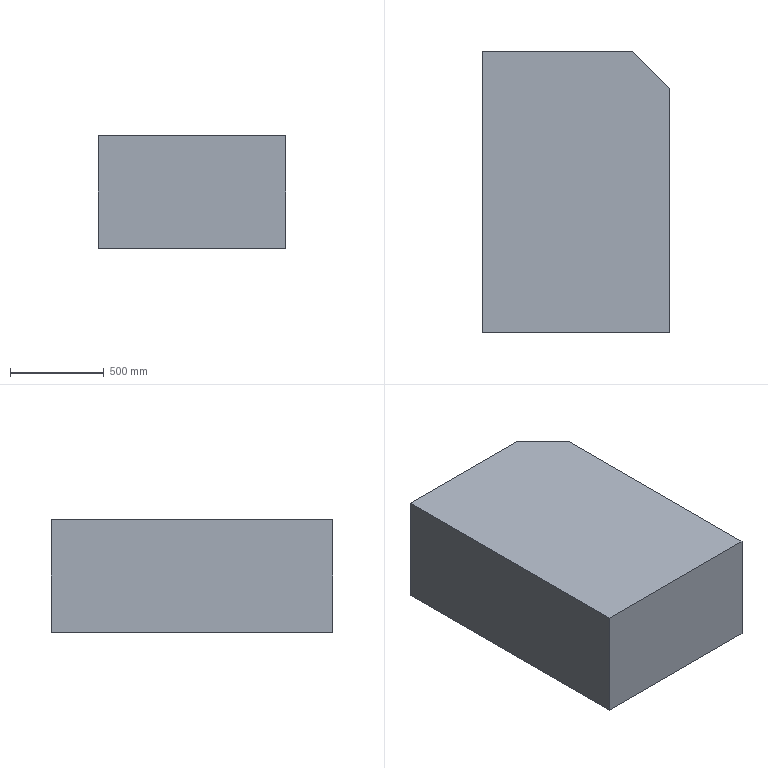Part | SolidWorks | features Chamfer 1, Extrusion 1 | 1 solid | 7 faces | box 1000 x 1500 x 600 mm | volume 888000000 mm3 | plane 7
STEP:
#1=CARTESIAN_POINT('',(500.,-750.,0.));
#2=VERTEX_POINT('',#1);
#3=CARTESIAN_POINT('',(500.,550.,0.));
#4=VERTEX_POINT('',#3);
#5=CARTESIAN_POINT('',(500.,750.,0.));
#6=DIRECTION('',(0.,1.,0.));
#7=VECTOR('',#6,1000.);
#8=LINE('',#5,#7);
#9=EDGE_CURVE('',#2,#4,#8,.T.);
#10=ORIENTED_EDGE('',*,*,#9,.T.);
#11=CARTESIAN_POINT('',(500.,550.,600.));
#12=VERTEX_POINT('',#11);
#13=CARTESIAN_POINT('',(500.,550.,600.));
#14=DIRECTION('',(0.,0.,1.));
#15=VECTOR('',#14,1000.);
#16=LINE('',#13,#15);
#17=EDGE_CURVE('',#4,#12,#16,.T.);
#18=ORIENTED_EDGE('',*,*,#17,.T.);
#19=CARTESIAN_POINT('',(500.,-750.,600.));
#20=VERTEX_POINT('',#19);
#21=CARTESIAN_POINT('',(500.,750.,600.));
#22=DIRECTION('',(0.,1.,0.));
#23=VECTOR('',#22,1000.);
#24=LINE('',#21,#23);
#25=EDGE_CURVE('',#20,#12,#24,.T.);
#26=ORIENTED_EDGE('',*,*,#25,.F.);
#27=CARTESIAN_POINT('',(500.,-750.,600.));
#28=DIRECTION('',(0.,0.,-1.));
#29=VECTOR('',#28,1000.);
#30=LINE('',#27,#29);
#31=EDGE_CURVE('',#20,#2,#30,.T.);
#32=ORIENTED_EDGE('',*,*,#31,.T.);
#33=EDGE_LOOP('',(#10,#18,#26,#32));
#34=FACE_OUTER_BOUND('',#33,.T.);
#35=CARTESIAN_POINT('',(500.,750.,600.));
#36=DIRECTION('',(-1.,0.,0.));
#37=DIRECTION('',(0.,-1.,0.));
#38=AXIS2_PLACEMENT_3D('',#35,#36,#37);
#39=PLANE('',#38);
#40=ADVANCED_FACE('',(#34),#39,.F.);
#41=CARTESIAN_POINT('',(300.,750.,600.));
#42=VERTEX_POINT('',#41);
#43=CARTESIAN_POINT('',(-500.,750.,600.));
#44=VERTEX_POINT('',#43);
#45=CARTESIAN_POINT('',(-500.,750.,600.));
#46=DIRECTION('',(-1.,0.,0.));
#47=VECTOR('',#46,1000.);
#48=LINE('',#45,#47);
#49=EDGE_CURVE('',#42,#44,#48,.T.);
#50=ORIENTED_EDGE('',*,*,#49,.F.);
#51=CARTESIAN_POINT('',(300.,750.,0.));
#52=VERTEX_POINT('',#51);
#53=CARTESIAN_POINT('',(300.,750.,600.));
#54=DIRECTION('',(0.,0.,-1.));
#55=VECTOR('',#54,1000.);
#56=LINE('',#53,#55);
#57=EDGE_CURVE('',#42,#52,#56,.T.);
#58=ORIENTED_EDGE('',*,*,#57,.T.);
#59=CARTESIAN_POINT('',(-500.,750.,0.));
#60=VERTEX_POINT('',#59);
#61=CARTESIAN_POINT('',(-500.,750.,0.));
#62=DIRECTION('',(-1.,0.,0.));
#63=VECTOR('',#62,1000.);
#64=LINE('',#61,#63);
#65=EDGE_CURVE('',#52,#60,#64,.T.);
#66=ORIENTED_EDGE('',*,*,#65,.T.);
#67=CARTESIAN_POINT('',(-500.,750.,600.));
#68=DIRECTION('',(0.,0.,-1.));
#69=VECTOR('',#68,1000.);
#70=LINE('',#67,#69);
#71=EDGE_CURVE('',#44,#60,#70,.T.);
#72=ORIENTED_EDGE('',*,*,#71,.F.);
#73=EDGE_LOOP('',(#50,#58,#66,#72));
#74=FACE_OUTER_BOUND('',#73,.T.);
#75=CARTESIAN_POINT('',(-500.,750.,600.));
#76=DIRECTION('',(0.,-1.,0.));
#77=DIRECTION('',(0.,0.,-1.));
#78=AXIS2_PLACEMENT_3D('',#75,#76,#77);
#79=PLANE('',#78);
#80=ADVANCED_FACE('',(#74),#79,.F.);
#81=CARTESIAN_POINT('',(-500.,-750.,0.));
#82=VERTEX_POINT('',#81);
#83=CARTESIAN_POINT('',(-500.,750.,0.));
#84=DIRECTION('',(0.,-1.,0.));
#85=VECTOR('',#84,1000.);
#86=LINE('',#83,#85);
#87=EDGE_CURVE('',#60,#82,#86,.T.);
#88=ORIENTED_EDGE('',*,*,#87,.T.);
#89=CARTESIAN_POINT('',(-500.,-750.,600.));
#90=VERTEX_POINT('',#89);
#91=CARTESIAN_POINT('',(-500.,-750.,600.));
#92=DIRECTION('',(0.,0.,-1.));
#93=VECTOR('',#92,1000.);
#94=LINE('',#91,#93);
#95=EDGE_CURVE('',#90,#82,#94,.T.);
#96=ORIENTED_EDGE('',*,*,#95,.F.);
#97=CARTESIAN_POINT('',(-500.,750.,600.));
#98=DIRECTION('',(0.,-1.,0.));
#99=VECTOR('',#98,1000.);
#100=LINE('',#97,#99);
#101=EDGE_CURVE('',#44,#90,#100,.T.);
#102=ORIENTED_EDGE('',*,*,#101,.F.);
#103=ORIENTED_EDGE('',*,*,#71,.T.);
#104=EDGE_LOOP('',(#88,#96,#102,#103));
#105=FACE_OUTER_BOUND('',#104,.T.);
#106=CARTESIAN_POINT('',(-500.,750.,600.));
#107=DIRECTION('',(1.,0.,0.));
#108=DIRECTION('',(0.,1.,0.));
#109=AXIS2_PLACEMENT_3D('',#106,#107,#108);
#110=PLANE('',#109);
#111=ADVANCED_FACE('',(#105),#110,.F.);
#112=CARTESIAN_POINT('',(-500.,-750.,0.));
#113=DIRECTION('',(1.,0.,0.));
#114=VECTOR('',#113,1000.);
#115=LINE('',#112,#114);
#116=EDGE_CURVE('',#82,#2,#115,.T.);
#117=ORIENTED_EDGE('',*,*,#116,.T.);
#118=ORIENTED_EDGE('',*,*,#31,.F.);
#119=CARTESIAN_POINT('',(-500.,-750.,600.));
#120=DIRECTION('',(1.,0.,0.));
#121=VECTOR('',#120,1000.);
#122=LINE('',#119,#121);
#123=EDGE_CURVE('',#90,#20,#122,.T.);
#124=ORIENTED_EDGE('',*,*,#123,.F.);
#125=ORIENTED_EDGE('',*,*,#95,.T.);
#126=EDGE_LOOP('',(#117,#118,#124,#125));
#127=FACE_OUTER_BOUND('',#126,.T.);
#128=CARTESIAN_POINT('',(-500.,-750.,600.));
#129=DIRECTION('',(0.,1.,0.));
#130=DIRECTION('',(0.,0.,1.));
#131=AXIS2_PLACEMENT_3D('',#128,#129,#130);
#132=PLANE('',#131);
#133=ADVANCED_FACE('',(#127),#132,.F.);
#134=ORIENTED_EDGE('',*,*,#25,.T.);
#135=CARTESIAN_POINT('',(525.,525.,600.));
#136=DIRECTION('',(-0.7071,0.7071,0.));
#137=VECTOR('',#136,1000.);
#138=LINE('',#135,#137);
#139=EDGE_CURVE('',#12,#42,#138,.T.);
#140=ORIENTED_EDGE('',*,*,#139,.T.);
#141=ORIENTED_EDGE('',*,*,#49,.T.);
#142=ORIENTED_EDGE('',*,*,#101,.T.);
#143=ORIENTED_EDGE('',*,*,#123,.T.);
#144=EDGE_LOOP('',(#134,#140,#141,#142,#143));
#145=FACE_OUTER_BOUND('',#144,.T.);
#146=CARTESIAN_POINT('',(0.,0.,600.));
#147=DIRECTION('',(0.,0.,1.));
#148=DIRECTION('',(1.,0.,0.));
#149=AXIS2_PLACEMENT_3D('',#146,#147,#148);
#150=PLANE('',#149);
#151=ADVANCED_FACE('',(#145),#150,.T.);
#152=ORIENTED_EDGE('',*,*,#65,.F.);
#153=CARTESIAN_POINT('',(300.,750.,0.));
#154=DIRECTION('',(0.7071,-0.7071,0.));
#155=VECTOR('',#154,1000.);
#156=LINE('',#153,#155);
#157=EDGE_CURVE('',#52,#4,#156,.T.);
#158=ORIENTED_EDGE('',*,*,#157,.T.);
#159=ORIENTED_EDGE('',*,*,#9,.F.);
#160=ORIENTED_EDGE('',*,*,#116,.F.);
#161=ORIENTED_EDGE('',*,*,#87,.F.);
#162=EDGE_LOOP('',(#152,#158,#159,#160,#161));
#163=FACE_OUTER_BOUND('',#162,.T.);
#164=CARTESIAN_POINT('',(0.,0.,0.));
#165=DIRECTION('',(0.,0.,1.));
#166=DIRECTION('',(1.,0.,0.));
#167=AXIS2_PLACEMENT_3D('',#164,#165,#166);
#168=PLANE('',#167);
#169=ADVANCED_FACE('',(#163),#168,.F.);
#170=ORIENTED_EDGE('',*,*,#139,.F.);
#171=ORIENTED_EDGE('',*,*,#17,.F.);
#172=ORIENTED_EDGE('',*,*,#157,.F.);
#173=ORIENTED_EDGE('',*,*,#57,.F.);
#174=EDGE_LOOP('',(#170,#171,#172,#173));
#175=FACE_OUTER_BOUND('',#174,.T.);
#176=CARTESIAN_POINT('',(300.,750.,600.));
#177=DIRECTION('',(-0.7071,-0.7071,0.));
#178=DIRECTION('',(0.,0.,-1.));
#179=AXIS2_PLACEMENT_3D('',#176,#177,#178);
#180=PLANE('',#179);
#181=ADVANCED_FACE('',(#175),#180,.F.);
#182=CLOSED_SHELL('',(#40,#80,#111,#133,#151,#169,#181));
#183=MANIFOLD_SOLID_BREP('',#182);
#184=CARTESIAN_POINT('',(0.,0.,0.));
#185=DIRECTION('',(0.,0.,1.));
#186=DIRECTION('',(1.,0.,0.));
#187=AXIS2_PLACEMENT_3D('',#184,#185,#186);
#188=(LENGTH_UNIT()NAMED_UNIT(*)SI_UNIT(.MILLI.,.METRE.));
#189=UNCERTAINTY_MEASURE_WITH_UNIT(LENGTH_MEASURE(0.00001),#188,'','');
#190=(NAMED_UNIT(*)PLANE_ANGLE_UNIT()SI_UNIT($,.RADIAN.));
#191=(NAMED_UNIT(*)SI_UNIT($,.STERADIAN.)SOLID_ANGLE_UNIT());
#192=(GEOMETRIC_REPRESENTATION_CONTEXT(3)GLOBAL_UNCERTAINTY_ASSIGNED_CONTEXT((#189))GLOBAL_UNIT_ASSIGNED_CONTEXT((#188,#190,#191))REPRESENTATION_CONTEXT('',''));
#193=ADVANCED_BREP_SHAPE_REPRESENTATION('',(#183,#187),#192);